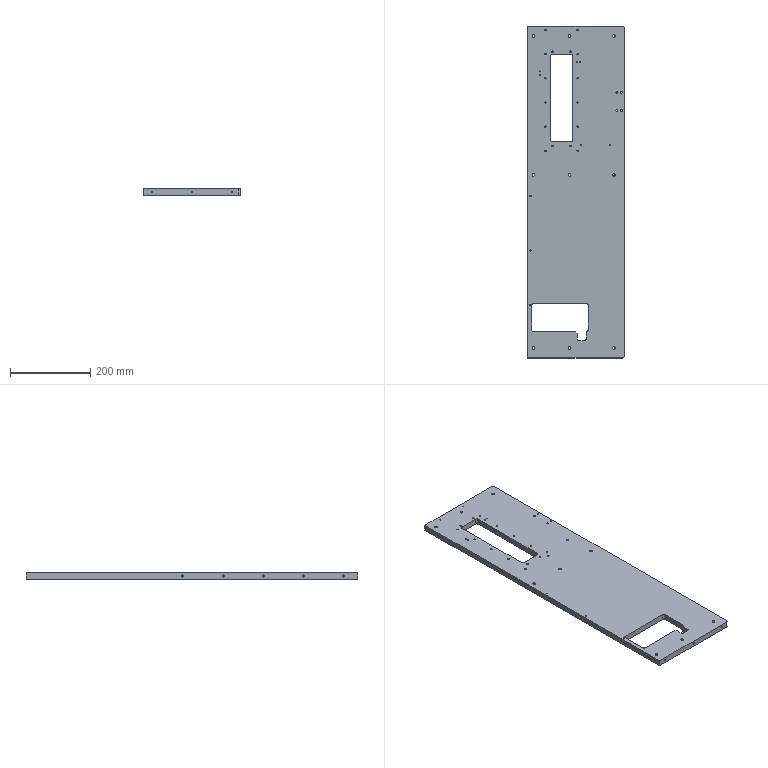Part | NX | features BREP 1 | 1 solid | 333 faces | box 240 x 825 x 15 mm | volume 2535496 mm3 | cylinder 194 | cone 101 | plane 38 | commonest cylinder face diameters 3.3 x84 2.5 x28 6.6 x18 14 x18 4.2 x16 5 x10